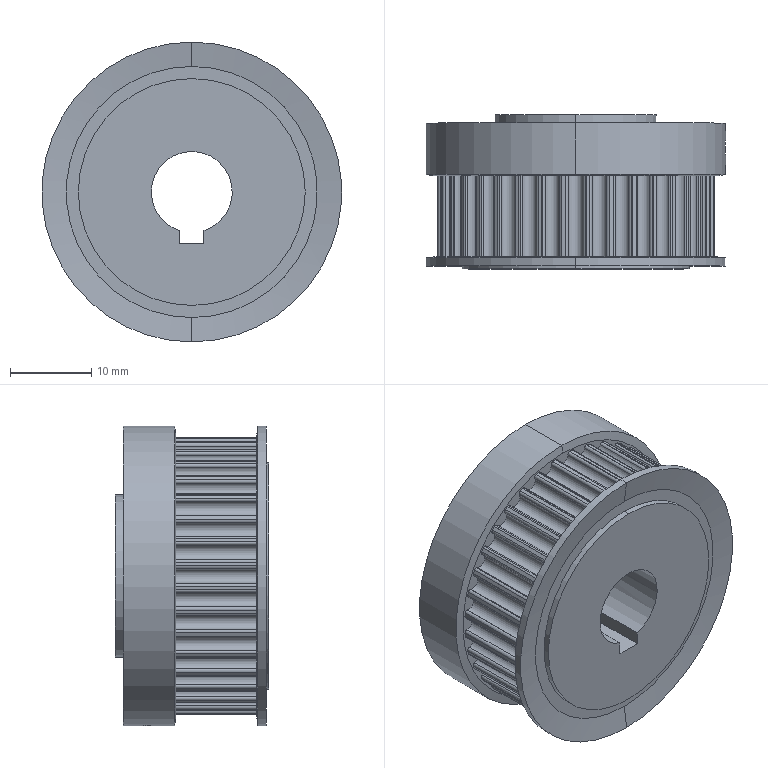Part | STEP file | 36-3M-φ10-19-J timing pulley | 1 solid | 280 faces | box 37 x 19 x 37 mm | volume 15386 mm3 | cylinder 193 | plane 81 | cone 6 | commonest cylinder face diameters 0.665 x90 1.8 x53 34.22 x36 2.5 x4 37 x4 10 x2